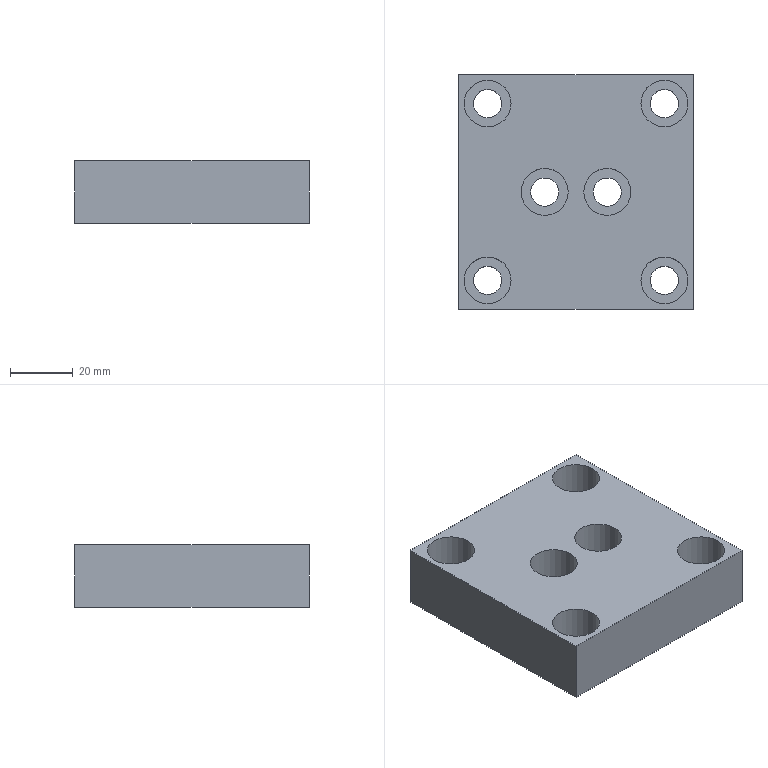Part | NX | features solid 2 | 1 solid | 24 faces | box 75 x 75 x 20 mm | volume 96271 mm3 | plane 12 | cylinder 12 | commonest cylinder face diameters 9 x6 15 x6
STEP:
#1=CARTESIAN_POINT('',(8.75,-278.25,320.));
#2=VERTEX_POINT('',#1);
#3=CARTESIAN_POINT('',(13.25,-278.25,320.));
#4=DIRECTION('',(0.,0.,-1.));
#5=DIRECTION('',(-1.,0.,0.));
#6=AXIS2_PLACEMENT_3D('',#3,#4,#5);
#7=CIRCLE('',#6,4.5);
#8=EDGE_CURVE('',#2,#2,#7,.F.);
#9=ORIENTED_EDGE('',*,*,#8,.T.);
#10=EDGE_LOOP('',(#9));
#11=FACE_BOUND('',#10,.T.);
#12=CARTESIAN_POINT('',(8.75,-221.75,320.));
#13=VERTEX_POINT('',#12);
#14=CARTESIAN_POINT('',(13.25,-221.75,320.));
#15=DIRECTION('',(0.,0.,-1.));
#16=DIRECTION('',(-1.,0.,0.));
#17=AXIS2_PLACEMENT_3D('',#14,#15,#16);
#18=CIRCLE('',#17,4.5);
#19=EDGE_CURVE('',#13,#13,#18,.F.);
#20=ORIENTED_EDGE('',*,*,#19,.T.);
#21=EDGE_LOOP('',(#20));
#22=FACE_BOUND('',#21,.T.);
#23=CARTESIAN_POINT('',(-47.75,-278.25,320.));
#24=VERTEX_POINT('',#23);
#25=CARTESIAN_POINT('',(-43.25,-278.25,320.));
#26=DIRECTION('',(0.,0.,-1.));
#27=DIRECTION('',(-1.,0.,0.));
#28=AXIS2_PLACEMENT_3D('',#25,#26,#27);
#29=CIRCLE('',#28,4.5);
#30=EDGE_CURVE('',#24,#24,#29,.F.);
#31=ORIENTED_EDGE('',*,*,#30,.T.);
#32=EDGE_LOOP('',(#31));
#33=FACE_BOUND('',#32,.T.);
#34=CARTESIAN_POINT('',(-47.75,-221.75,320.));
#35=VERTEX_POINT('',#34);
#36=CARTESIAN_POINT('',(-43.25,-221.75,320.));
#37=DIRECTION('',(0.,0.,-1.));
#38=DIRECTION('',(-1.,0.,0.));
#39=AXIS2_PLACEMENT_3D('',#36,#37,#38);
#40=CIRCLE('',#39,4.5);
#41=EDGE_CURVE('',#35,#35,#40,.F.);
#42=ORIENTED_EDGE('',*,*,#41,.T.);
#43=EDGE_LOOP('',(#42));
#44=FACE_BOUND('',#43,.T.);
#45=CARTESIAN_POINT('',(-9.5,-250.,320.));
#46=VERTEX_POINT('',#45);
#47=CARTESIAN_POINT('',(-5.,-250.,320.));
#48=DIRECTION('',(0.,0.,-1.));
#49=DIRECTION('',(-1.,0.,0.));
#50=AXIS2_PLACEMENT_3D('',#47,#48,#49);
#51=CIRCLE('',#50,4.5);
#52=EDGE_CURVE('',#46,#46,#51,.F.);
#53=ORIENTED_EDGE('',*,*,#52,.T.);
#54=EDGE_LOOP('',(#53));
#55=FACE_BOUND('',#54,.T.);
#56=CARTESIAN_POINT('',(-29.5,-250.,320.));
#57=VERTEX_POINT('',#56);
#58=CARTESIAN_POINT('',(-25.,-250.,320.));
#59=DIRECTION('',(0.,0.,-1.));
#60=DIRECTION('',(-1.,0.,0.));
#61=AXIS2_PLACEMENT_3D('',#58,#59,#60);
#62=CIRCLE('',#61,4.5);
#63=EDGE_CURVE('',#57,#57,#62,.F.);
#64=ORIENTED_EDGE('',*,*,#63,.T.);
#65=EDGE_LOOP('',(#64));
#66=FACE_BOUND('',#65,.T.);
#67=CARTESIAN_POINT('',(-52.5,-212.5,320.));
#68=VERTEX_POINT('',#67);
#69=CARTESIAN_POINT('',(22.5,-212.5,320.));
#70=VERTEX_POINT('',#69);
#71=CARTESIAN_POINT('',(-52.5,-212.5,320.));
#72=DIRECTION('',(-1.,0.,0.));
#73=VECTOR('',#72,1000.);
#74=LINE('',#71,#73);
#75=EDGE_CURVE('',#68,#70,#74,.F.);
#76=ORIENTED_EDGE('',*,*,#75,.T.);
#77=CARTESIAN_POINT('',(22.5,-287.5,320.));
#78=VERTEX_POINT('',#77);
#79=CARTESIAN_POINT('',(22.5,-212.5,320.));
#80=DIRECTION('',(0.,1.,0.));
#81=VECTOR('',#80,1000.);
#82=LINE('',#79,#81);
#83=EDGE_CURVE('',#70,#78,#82,.F.);
#84=ORIENTED_EDGE('',*,*,#83,.T.);
#85=CARTESIAN_POINT('',(-52.5,-287.5,320.));
#86=VERTEX_POINT('',#85);
#87=CARTESIAN_POINT('',(-52.5,-287.5,320.));
#88=DIRECTION('',(-1.,0.,0.));
#89=VECTOR('',#88,1000.);
#90=LINE('',#87,#89);
#91=EDGE_CURVE('',#86,#78,#90,.F.);
#92=ORIENTED_EDGE('',*,*,#91,.F.);
#93=CARTESIAN_POINT('',(-52.5,-212.5,320.));
#94=DIRECTION('',(0.,-1.,0.));
#95=VECTOR('',#94,1000.);
#96=LINE('',#93,#95);
#97=EDGE_CURVE('',#68,#86,#96,.T.);
#98=ORIENTED_EDGE('',*,*,#97,.F.);
#99=EDGE_LOOP('',(#76,#84,#92,#98));
#100=FACE_BOUND('',#99,.T.);
#101=CARTESIAN_POINT('',(-52.5,-212.5,320.));
#102=DIRECTION('',(0.,0.,-1.));
#103=DIRECTION('',(0.,-1.,0.));
#104=AXIS2_PLACEMENT_3D('',#101,#102,#103);
#105=PLANE('',#104);
#106=ADVANCED_FACE('',(#11,#22,#33,#44,#55,#66,#100),#105,.T.);
#107=ORIENTED_EDGE('',*,*,#91,.T.);
#108=CARTESIAN_POINT('',(22.5,-287.5,340.));
#109=VERTEX_POINT('',#108);
#110=CARTESIAN_POINT('',(22.5,-287.5,320.));
#111=DIRECTION('',(0.,0.,1.));
#112=VECTOR('',#111,1000.);
#113=LINE('',#110,#112);
#114=EDGE_CURVE('',#78,#109,#113,.T.);
#115=ORIENTED_EDGE('',*,*,#114,.T.);
#116=CARTESIAN_POINT('',(-52.5,-287.5,340.));
#117=VERTEX_POINT('',#116);
#118=CARTESIAN_POINT('',(-52.5,-287.5,340.));
#119=DIRECTION('',(-1.,0.,0.));
#120=VECTOR('',#119,1000.);
#121=LINE('',#118,#120);
#122=EDGE_CURVE('',#117,#109,#121,.F.);
#123=ORIENTED_EDGE('',*,*,#122,.F.);
#124=CARTESIAN_POINT('',(-52.5,-287.5,320.));
#125=DIRECTION('',(0.,0.,1.));
#126=VECTOR('',#125,1000.);
#127=LINE('',#124,#126);
#128=EDGE_CURVE('',#86,#117,#127,.T.);
#129=ORIENTED_EDGE('',*,*,#128,.F.);
#130=EDGE_LOOP('',(#107,#115,#123,#129));
#131=FACE_BOUND('',#130,.T.);
#132=CARTESIAN_POINT('',(-52.5,-287.5,320.));
#133=DIRECTION('',(0.,-1.,0.));
#134=DIRECTION('',(0.,0.,1.));
#135=AXIS2_PLACEMENT_3D('',#132,#133,#134);
#136=PLANE('',#135);
#137=ADVANCED_FACE('',(#131),#136,.T.);
#138=CARTESIAN_POINT('',(5.75,-278.25,340.));
#139=VERTEX_POINT('',#138);
#140=CARTESIAN_POINT('',(13.25,-278.25,340.));
#141=DIRECTION('',(0.,0.,-1.));
#142=DIRECTION('',(-1.,0.,0.));
#143=AXIS2_PLACEMENT_3D('',#140,#141,#142);
#144=CIRCLE('',#143,7.5);
#145=EDGE_CURVE('',#139,#139,#144,.T.);
#146=ORIENTED_EDGE('',*,*,#145,.T.);
#147=EDGE_LOOP('',(#146));
#148=FACE_BOUND('',#147,.T.);
#149=CARTESIAN_POINT('',(5.75,-221.75,340.));
#150=VERTEX_POINT('',#149);
#151=CARTESIAN_POINT('',(13.25,-221.75,340.));
#152=DIRECTION('',(0.,0.,-1.));
#153=DIRECTION('',(-1.,0.,0.));
#154=AXIS2_PLACEMENT_3D('',#151,#152,#153);
#155=CIRCLE('',#154,7.5);
#156=EDGE_CURVE('',#150,#150,#155,.T.);
#157=ORIENTED_EDGE('',*,*,#156,.T.);
#158=EDGE_LOOP('',(#157));
#159=FACE_BOUND('',#158,.T.);
#160=CARTESIAN_POINT('',(-50.75,-278.25,340.));
#161=VERTEX_POINT('',#160);
#162=CARTESIAN_POINT('',(-43.25,-278.25,340.));
#163=DIRECTION('',(0.,0.,-1.));
#164=DIRECTION('',(-1.,0.,0.));
#165=AXIS2_PLACEMENT_3D('',#162,#163,#164);
#166=CIRCLE('',#165,7.5);
#167=EDGE_CURVE('',#161,#161,#166,.T.);
#168=ORIENTED_EDGE('',*,*,#167,.T.);
#169=EDGE_LOOP('',(#168));
#170=FACE_BOUND('',#169,.T.);
#171=CARTESIAN_POINT('',(-50.75,-221.75,340.));
#172=VERTEX_POINT('',#171);
#173=CARTESIAN_POINT('',(-43.25,-221.75,340.));
#174=DIRECTION('',(0.,0.,-1.));
#175=DIRECTION('',(-1.,0.,0.));
#176=AXIS2_PLACEMENT_3D('',#173,#174,#175);
#177=CIRCLE('',#176,7.5);
#178=EDGE_CURVE('',#172,#172,#177,.T.);
#179=ORIENTED_EDGE('',*,*,#178,.T.);
#180=EDGE_LOOP('',(#179));
#181=FACE_BOUND('',#180,.T.);
#182=CARTESIAN_POINT('',(-12.5,-250.,340.));
#183=VERTEX_POINT('',#182);
#184=CARTESIAN_POINT('',(-5.,-250.,340.));
#185=DIRECTION('',(0.,0.,-1.));
#186=DIRECTION('',(-1.,0.,0.));
#187=AXIS2_PLACEMENT_3D('',#184,#185,#186);
#188=CIRCLE('',#187,7.5);
#189=EDGE_CURVE('',#183,#183,#188,.T.);
#190=ORIENTED_EDGE('',*,*,#189,.T.);
#191=EDGE_LOOP('',(#190));
#192=FACE_BOUND('',#191,.T.);
#193=CARTESIAN_POINT('',(-32.5,-250.,340.));
#194=VERTEX_POINT('',#193);
#195=CARTESIAN_POINT('',(-25.,-250.,340.));
#196=DIRECTION('',(0.,0.,-1.));
#197=DIRECTION('',(-1.,0.,0.));
#198=AXIS2_PLACEMENT_3D('',#195,#196,#197);
#199=CIRCLE('',#198,7.5);
#200=EDGE_CURVE('',#194,#194,#199,.T.);
#201=ORIENTED_EDGE('',*,*,#200,.T.);
#202=EDGE_LOOP('',(#201));
#203=FACE_BOUND('',#202,.T.);
#204=ORIENTED_EDGE('',*,*,#122,.T.);
#205=CARTESIAN_POINT('',(22.5,-212.5,340.));
#206=VERTEX_POINT('',#205);
#207=CARTESIAN_POINT('',(22.5,-212.5,340.));
#208=DIRECTION('',(0.,-1.,0.));
#209=VECTOR('',#208,1000.);
#210=LINE('',#207,#209);
#211=EDGE_CURVE('',#206,#109,#210,.T.);
#212=ORIENTED_EDGE('',*,*,#211,.F.);
#213=CARTESIAN_POINT('',(-52.5,-212.5,340.));
#214=VERTEX_POINT('',#213);
#215=CARTESIAN_POINT('',(-52.5,-212.5,340.));
#216=DIRECTION('',(1.,0.,0.));
#217=VECTOR('',#216,1000.);
#218=LINE('',#215,#217);
#219=EDGE_CURVE('',#214,#206,#218,.T.);
#220=ORIENTED_EDGE('',*,*,#219,.F.);
#221=CARTESIAN_POINT('',(-52.5,-212.5,340.));
#222=DIRECTION('',(0.,-1.,0.));
#223=VECTOR('',#222,1000.);
#224=LINE('',#221,#223);
#225=EDGE_CURVE('',#214,#117,#224,.T.);
#226=ORIENTED_EDGE('',*,*,#225,.T.);
#227=EDGE_LOOP('',(#204,#212,#220,#226));
#228=FACE_BOUND('',#227,.T.);
#229=CARTESIAN_POINT('',(-52.5,-212.5,340.));
#230=DIRECTION('',(0.,0.,-1.));
#231=DIRECTION('',(0.,-1.,0.));
#232=AXIS2_PLACEMENT_3D('',#229,#230,#231);
#233=PLANE('',#232);
#234=ADVANCED_FACE('',(#148,#159,#170,#181,#192,#203,#228),#233,.F.);
#235=CARTESIAN_POINT('',(-52.5,-212.5,320.));
#236=DIRECTION('',(0.,0.,1.));
#237=VECTOR('',#236,1000.);
#238=LINE('',#235,#237);
#239=EDGE_CURVE('',#68,#214,#238,.T.);
#240=ORIENTED_EDGE('',*,*,#239,.T.);
#241=ORIENTED_EDGE('',*,*,#219,.T.);
#242=CARTESIAN_POINT('',(22.5,-212.5,320.));
#243=DIRECTION('',(0.,0.,1.));
#244=VECTOR('',#243,1000.);
#245=LINE('',#242,#244);
#246=EDGE_CURVE('',#70,#206,#245,.T.);
#247=ORIENTED_EDGE('',*,*,#246,.F.);
#248=ORIENTED_EDGE('',*,*,#75,.F.);
#249=EDGE_LOOP('',(#240,#241,#247,#248));
#250=FACE_BOUND('',#249,.T.);
#251=CARTESIAN_POINT('',(-52.5,-212.5,320.));
#252=DIRECTION('',(0.,-1.,0.));
#253=DIRECTION('',(0.,0.,1.));
#254=AXIS2_PLACEMENT_3D('',#251,#252,#253);
#255=PLANE('',#254);
#256=ADVANCED_FACE('',(#250),#255,.F.);
#257=ORIENTED_EDGE('',*,*,#211,.T.);
#258=ORIENTED_EDGE('',*,*,#114,.F.);
#259=ORIENTED_EDGE('',*,*,#83,.F.);
#260=ORIENTED_EDGE('',*,*,#246,.T.);
#261=EDGE_LOOP('',(#257,#258,#259,#260));
#262=FACE_BOUND('',#261,.T.);
#263=CARTESIAN_POINT('',(22.5,-212.5,320.));
#264=DIRECTION('',(-1.,0.,0.));
#265=DIRECTION('',(0.,0.,1.));
#266=AXIS2_PLACEMENT_3D('',#263,#264,#265);
#267=PLANE('',#266);
#268=ADVANCED_FACE('',(#262),#267,.F.);
#269=ORIENTED_EDGE('',*,*,#225,.F.);
#270=ORIENTED_EDGE('',*,*,#239,.F.);
#271=ORIENTED_EDGE('',*,*,#97,.T.);
#272=ORIENTED_EDGE('',*,*,#128,.T.);
#273=EDGE_LOOP('',(#269,#270,#271,#272));
#274=FACE_BOUND('',#273,.T.);
#275=CARTESIAN_POINT('',(-52.5,-212.5,320.));
#276=DIRECTION('',(-1.,0.,0.));
#277=DIRECTION('',(0.,0.,1.));
#278=AXIS2_PLACEMENT_3D('',#275,#276,#277);
#279=PLANE('',#278);
#280=ADVANCED_FACE('',(#274),#279,.T.);
#281=CARTESIAN_POINT('',(-29.5,-250.,326.));
#282=VERTEX_POINT('',#281);
#283=CARTESIAN_POINT('',(-25.,-250.,326.));
#284=DIRECTION('',(0.,0.,-1.));
#285=DIRECTION('',(-1.,0.,0.));
#286=AXIS2_PLACEMENT_3D('',#283,#284,#285);
#287=CIRCLE('',#286,4.5);
#288=EDGE_CURVE('',#282,#282,#287,.T.);
#289=ORIENTED_EDGE('',*,*,#288,.F.);
#290=EDGE_LOOP('',(#289));
#291=FACE_BOUND('',#290,.T.);
#292=ORIENTED_EDGE('',*,*,#63,.F.);
#293=EDGE_LOOP('',(#292));
#294=FACE_BOUND('',#293,.T.);
#295=CARTESIAN_POINT('',(-25.,-250.,290.));
#296=DIRECTION('',(0.,0.,-1.));
#297=DIRECTION('',(-1.,0.,0.));
#298=AXIS2_PLACEMENT_3D('',#295,#296,#297);
#299=CYLINDRICAL_SURFACE('',#298,4.5);
#300=ADVANCED_FACE('',(#291,#294),#299,.F.);
#301=ORIENTED_EDGE('',*,*,#288,.T.);
#302=EDGE_LOOP('',(#301));
#303=FACE_BOUND('',#302,.T.);
#304=CARTESIAN_POINT('',(-32.5,-250.,326.));
#305=VERTEX_POINT('',#304);
#306=CARTESIAN_POINT('',(-25.,-250.,326.));
#307=DIRECTION('',(0.,0.,-1.));
#308=DIRECTION('',(-1.,0.,0.));
#309=AXIS2_PLACEMENT_3D('',#306,#307,#308);
#310=CIRCLE('',#309,7.5);
#311=EDGE_CURVE('',#305,#305,#310,.T.);
#312=ORIENTED_EDGE('',*,*,#311,.F.);
#313=EDGE_LOOP('',(#312));
#314=FACE_BOUND('',#313,.T.);
#315=CARTESIAN_POINT('',(-25.,-250.,326.));
#316=DIRECTION('',(0.,0.,-1.));
#317=DIRECTION('',(-1.,0.,0.));
#318=AXIS2_PLACEMENT_3D('',#315,#316,#317);
#319=PLANE('',#318);
#320=ADVANCED_FACE('',(#303,#314),#319,.F.);
#321=ORIENTED_EDGE('',*,*,#311,.T.);
#322=EDGE_LOOP('',(#321));
#323=FACE_BOUND('',#322,.T.);
#324=ORIENTED_EDGE('',*,*,#200,.F.);
#325=EDGE_LOOP('',(#324));
#326=FACE_BOUND('',#325,.T.);
#327=CARTESIAN_POINT('',(-25.,-250.,340.));
#328=DIRECTION('',(0.,0.,-1.));
#329=DIRECTION('',(-1.,0.,0.));
#330=AXIS2_PLACEMENT_3D('',#327,#328,#329);
#331=CYLINDRICAL_SURFACE('',#330,7.5);
#332=ADVANCED_FACE('',(#323,#326),#331,.F.);
#333=CARTESIAN_POINT('',(-9.5,-250.,326.));
#334=VERTEX_POINT('',#333);
#335=CARTESIAN_POINT('',(-5.,-250.,326.));
#336=DIRECTION('',(0.,0.,-1.));
#337=DIRECTION('',(-1.,0.,0.));
#338=AXIS2_PLACEMENT_3D('',#335,#336,#337);
#339=CIRCLE('',#338,4.5);
#340=EDGE_CURVE('',#334,#334,#339,.T.);
#341=ORIENTED_EDGE('',*,*,#340,.F.);
#342=EDGE_LOOP('',(#341));
#343=FACE_BOUND('',#342,.T.);
#344=ORIENTED_EDGE('',*,*,#52,.F.);
#345=EDGE_LOOP('',(#344));
#346=FACE_BOUND('',#345,.T.);
#347=CARTESIAN_POINT('',(-5.,-250.,290.));
#348=DIRECTION('',(0.,0.,-1.));
#349=DIRECTION('',(-1.,0.,0.));
#350=AXIS2_PLACEMENT_3D('',#347,#348,#349);
#351=CYLINDRICAL_SURFACE('',#350,4.5);
#352=ADVANCED_FACE('',(#343,#346),#351,.F.);
#353=ORIENTED_EDGE('',*,*,#340,.T.);
#354=EDGE_LOOP('',(#353));
#355=FACE_BOUND('',#354,.T.);
#356=CARTESIAN_POINT('',(-12.5,-250.,326.));
#357=VERTEX_POINT('',#356);
#358=CARTESIAN_POINT('',(-5.,-250.,326.));
#359=DIRECTION('',(0.,0.,-1.));
#360=DIRECTION('',(-1.,0.,0.));
#361=AXIS2_PLACEMENT_3D('',#358,#359,#360);
#362=CIRCLE('',#361,7.5);
#363=EDGE_CURVE('',#357,#357,#362,.T.);
#364=ORIENTED_EDGE('',*,*,#363,.F.);
#365=EDGE_LOOP('',(#364));
#366=FACE_BOUND('',#365,.T.);
#367=CARTESIAN_POINT('',(-5.,-250.,326.));
#368=DIRECTION('',(0.,0.,-1.));
#369=DIRECTION('',(-1.,0.,0.));
#370=AXIS2_PLACEMENT_3D('',#367,#368,#369);
#371=PLANE('',#370);
#372=ADVANCED_FACE('',(#355,#366),#371,.F.);
#373=ORIENTED_EDGE('',*,*,#363,.T.);
#374=EDGE_LOOP('',(#373));
#375=FACE_BOUND('',#374,.T.);
#376=ORIENTED_EDGE('',*,*,#189,.F.);
#377=EDGE_LOOP('',(#376));
#378=FACE_BOUND('',#377,.T.);
#379=CARTESIAN_POINT('',(-5.,-250.,340.));
#380=DIRECTION('',(0.,0.,-1.));
#381=DIRECTION('',(-1.,0.,0.));
#382=AXIS2_PLACEMENT_3D('',#379,#380,#381);
#383=CYLINDRICAL_SURFACE('',#382,7.5);
#384=ADVANCED_FACE('',(#375,#378),#383,.F.);
#385=CARTESIAN_POINT('',(-47.75,-221.75,328.));
#386=VERTEX_POINT('',#385);
#387=CARTESIAN_POINT('',(-43.25,-221.75,328.));
#388=DIRECTION('',(0.,0.,-1.));
#389=DIRECTION('',(-1.,0.,0.));
#390=AXIS2_PLACEMENT_3D('',#387,#388,#389);
#391=CIRCLE('',#390,4.5);
#392=EDGE_CURVE('',#386,#386,#391,.T.);
#393=ORIENTED_EDGE('',*,*,#392,.F.);
#394=EDGE_LOOP('',(#393));
#395=FACE_BOUND('',#394,.T.);
#396=ORIENTED_EDGE('',*,*,#41,.F.);
#397=EDGE_LOOP('',(#396));
#398=FACE_BOUND('',#397,.T.);
#399=CARTESIAN_POINT('',(-43.25,-221.75,290.));
#400=DIRECTION('',(0.,0.,-1.));
#401=DIRECTION('',(-1.,0.,0.));
#402=AXIS2_PLACEMENT_3D('',#399,#400,#401);
#403=CYLINDRICAL_SURFACE('',#402,4.5);
#404=ADVANCED_FACE('',(#395,#398),#403,.F.);
#405=ORIENTED_EDGE('',*,*,#392,.T.);
#406=EDGE_LOOP('',(#405));
#407=FACE_BOUND('',#406,.T.);
#408=CARTESIAN_POINT('',(-50.75,-221.75,328.));
#409=VERTEX_POINT('',#408);
#410=CARTESIAN_POINT('',(-43.25,-221.75,328.));
#411=DIRECTION('',(0.,0.,-1.));
#412=DIRECTION('',(-1.,0.,0.));
#413=AXIS2_PLACEMENT_3D('',#410,#411,#412);
#414=CIRCLE('',#413,7.5);
#415=EDGE_CURVE('',#409,#409,#414,.T.);
#416=ORIENTED_EDGE('',*,*,#415,.F.);
#417=EDGE_LOOP('',(#416));
#418=FACE_BOUND('',#417,.T.);
#419=CARTESIAN_POINT('',(-43.25,-221.75,328.));
#420=DIRECTION('',(0.,0.,-1.));
#421=DIRECTION('',(-1.,0.,0.));
#422=AXIS2_PLACEMENT_3D('',#419,#420,#421);
#423=PLANE('',#422);
#424=ADVANCED_FACE('',(#407,#418),#423,.F.);
#425=ORIENTED_EDGE('',*,*,#415,.T.);
#426=EDGE_LOOP('',(#425));
#427=FACE_BOUND('',#426,.T.);
#428=ORIENTED_EDGE('',*,*,#178,.F.);
#429=EDGE_LOOP('',(#428));
#430=FACE_BOUND('',#429,.T.);
#431=CARTESIAN_POINT('',(-43.25,-221.75,340.));
#432=DIRECTION('',(0.,0.,-1.));
#433=DIRECTION('',(-1.,0.,0.));
#434=AXIS2_PLACEMENT_3D('',#431,#432,#433);
#435=CYLINDRICAL_SURFACE('',#434,7.5);
#436=ADVANCED_FACE('',(#427,#430),#435,.F.);
#437=CARTESIAN_POINT('',(-47.75,-278.25,328.));
#438=VERTEX_POINT('',#437);
#439=CARTESIAN_POINT('',(-43.25,-278.25,328.));
#440=DIRECTION('',(0.,0.,-1.));
#441=DIRECTION('',(-1.,0.,0.));
#442=AXIS2_PLACEMENT_3D('',#439,#440,#441);
#443=CIRCLE('',#442,4.5);
#444=EDGE_CURVE('',#438,#438,#443,.T.);
#445=ORIENTED_EDGE('',*,*,#444,.F.);
#446=EDGE_LOOP('',(#445));
#447=FACE_BOUND('',#446,.T.);
#448=ORIENTED_EDGE('',*,*,#30,.F.);
#449=EDGE_LOOP('',(#448));
#450=FACE_BOUND('',#449,.T.);
#451=CARTESIAN_POINT('',(-43.25,-278.25,290.));
#452=DIRECTION('',(0.,0.,-1.));
#453=DIRECTION('',(-1.,0.,0.));
#454=AXIS2_PLACEMENT_3D('',#451,#452,#453);
#455=CYLINDRICAL_SURFACE('',#454,4.5);
#456=ADVANCED_FACE('',(#447,#450),#455,.F.);
#457=ORIENTED_EDGE('',*,*,#444,.T.);
#458=EDGE_LOOP('',(#457));
#459=FACE_BOUND('',#458,.T.);
#460=CARTESIAN_POINT('',(-50.75,-278.25,328.));
#461=VERTEX_POINT('',#460);
#462=CARTESIAN_POINT('',(-43.25,-278.25,328.));
#463=DIRECTION('',(0.,0.,-1.));
#464=DIRECTION('',(-1.,0.,0.));
#465=AXIS2_PLACEMENT_3D('',#462,#463,#464);
#466=CIRCLE('',#465,7.5);
#467=EDGE_CURVE('',#461,#461,#466,.T.);
#468=ORIENTED_EDGE('',*,*,#467,.F.);
#469=EDGE_LOOP('',(#468));
#470=FACE_BOUND('',#469,.T.);
#471=CARTESIAN_POINT('',(-43.25,-278.25,328.));
#472=DIRECTION('',(0.,0.,-1.));
#473=DIRECTION('',(-1.,0.,0.));
#474=AXIS2_PLACEMENT_3D('',#471,#472,#473);
#475=PLANE('',#474);
#476=ADVANCED_FACE('',(#459,#470),#475,.F.);
#477=ORIENTED_EDGE('',*,*,#467,.T.);
#478=EDGE_LOOP('',(#477));
#479=FACE_BOUND('',#478,.T.);
#480=ORIENTED_EDGE('',*,*,#167,.F.);
#481=EDGE_LOOP('',(#480));
#482=FACE_BOUND('',#481,.T.);
#483=CARTESIAN_POINT('',(-43.25,-278.25,340.));
#484=DIRECTION('',(0.,0.,-1.));
#485=DIRECTION('',(-1.,0.,0.));
#486=AXIS2_PLACEMENT_3D('',#483,#484,#485);
#487=CYLINDRICAL_SURFACE('',#486,7.5);
#488=ADVANCED_FACE('',(#479,#482),#487,.F.);
#489=CARTESIAN_POINT('',(8.75,-221.75,328.));
#490=VERTEX_POINT('',#489);
#491=CARTESIAN_POINT('',(13.25,-221.75,328.));
#492=DIRECTION('',(0.,0.,-1.));
#493=DIRECTION('',(-1.,0.,0.));
#494=AXIS2_PLACEMENT_3D('',#491,#492,#493);
#495=CIRCLE('',#494,4.5);
#496=EDGE_CURVE('',#490,#490,#495,.T.);
#497=ORIENTED_EDGE('',*,*,#496,.F.);
#498=EDGE_LOOP('',(#497));
#499=FACE_BOUND('',#498,.T.);
#500=ORIENTED_EDGE('',*,*,#19,.F.);
#501=EDGE_LOOP('',(#500));
#502=FACE_BOUND('',#501,.T.);
#503=CARTESIAN_POINT('',(13.25,-221.75,290.));
#504=DIRECTION('',(0.,0.,-1.));
#505=DIRECTION('',(-1.,0.,0.));
#506=AXIS2_PLACEMENT_3D('',#503,#504,#505);
#507=CYLINDRICAL_SURFACE('',#506,4.5);
#508=ADVANCED_FACE('',(#499,#502),#507,.F.);
#509=ORIENTED_EDGE('',*,*,#496,.T.);
#510=EDGE_LOOP('',(#509));
#511=FACE_BOUND('',#510,.T.);
#512=CARTESIAN_POINT('',(5.75,-221.75,328.));
#513=VERTEX_POINT('',#512);
#514=CARTESIAN_POINT('',(13.25,-221.75,328.));
#515=DIRECTION('',(0.,0.,-1.));
#516=DIRECTION('',(-1.,0.,0.));
#517=AXIS2_PLACEMENT_3D('',#514,#515,#516);
#518=CIRCLE('',#517,7.5);
#519=EDGE_CURVE('',#513,#513,#518,.T.);
#520=ORIENTED_EDGE('',*,*,#519,.F.);
#521=EDGE_LOOP('',(#520));
#522=FACE_BOUND('',#521,.T.);
#523=CARTESIAN_POINT('',(13.25,-221.75,328.));
#524=DIRECTION('',(0.,0.,-1.));
#525=DIRECTION('',(-1.,0.,0.));
#526=AXIS2_PLACEMENT_3D('',#523,#524,#525);
#527=PLANE('',#526);
#528=ADVANCED_FACE('',(#511,#522),#527,.F.);
#529=ORIENTED_EDGE('',*,*,#519,.T.);
#530=EDGE_LOOP('',(#529));
#531=FACE_BOUND('',#530,.T.);
#532=ORIENTED_EDGE('',*,*,#156,.F.);
#533=EDGE_LOOP('',(#532));
#534=FACE_BOUND('',#533,.T.);
#535=CARTESIAN_POINT('',(13.25,-221.75,340.));
#536=DIRECTION('',(0.,0.,-1.));
#537=DIRECTION('',(-1.,0.,0.));
#538=AXIS2_PLACEMENT_3D('',#535,#536,#537);
#539=CYLINDRICAL_SURFACE('',#538,7.5);
#540=ADVANCED_FACE('',(#531,#534),#539,.F.);
#541=CARTESIAN_POINT('',(8.75,-278.25,328.));
#542=VERTEX_POINT('',#541);
#543=CARTESIAN_POINT('',(13.25,-278.25,328.));
#544=DIRECTION('',(0.,0.,-1.));
#545=DIRECTION('',(-1.,0.,0.));
#546=AXIS2_PLACEMENT_3D('',#543,#544,#545);
#547=CIRCLE('',#546,4.5);
#548=EDGE_CURVE('',#542,#542,#547,.T.);
#549=ORIENTED_EDGE('',*,*,#548,.F.);
#550=EDGE_LOOP('',(#549));
#551=FACE_BOUND('',#550,.T.);
#552=ORIENTED_EDGE('',*,*,#8,.F.);
#553=EDGE_LOOP('',(#552));
#554=FACE_BOUND('',#553,.T.);
#555=CARTESIAN_POINT('',(13.25,-278.25,290.));
#556=DIRECTION('',(0.,0.,-1.));
#557=DIRECTION('',(-1.,0.,0.));
#558=AXIS2_PLACEMENT_3D('',#555,#556,#557);
#559=CYLINDRICAL_SURFACE('',#558,4.5);
#560=ADVANCED_FACE('',(#551,#554),#559,.F.);
#561=ORIENTED_EDGE('',*,*,#548,.T.);
#562=EDGE_LOOP('',(#561));
#563=FACE_BOUND('',#562,.T.);
#564=CARTESIAN_POINT('',(5.75,-278.25,328.));
#565=VERTEX_POINT('',#564);
#566=CARTESIAN_POINT('',(13.25,-278.25,328.));
#567=DIRECTION('',(0.,0.,-1.));
#568=DIRECTION('',(-1.,0.,0.));
#569=AXIS2_PLACEMENT_3D('',#566,#567,#568);
#570=CIRCLE('',#569,7.5);
#571=EDGE_CURVE('',#565,#565,#570,.T.);
#572=ORIENTED_EDGE('',*,*,#571,.F.);
#573=EDGE_LOOP('',(#572));
#574=FACE_BOUND('',#573,.T.);
#575=CARTESIAN_POINT('',(13.25,-278.25,328.));
#576=DIRECTION('',(0.,0.,-1.));
#577=DIRECTION('',(-1.,0.,0.));
#578=AXIS2_PLACEMENT_3D('',#575,#576,#577);
#579=PLANE('',#578);
#580=ADVANCED_FACE('',(#563,#574),#579,.F.);
#581=ORIENTED_EDGE('',*,*,#571,.T.);
#582=EDGE_LOOP('',(#581));
#583=FACE_BOUND('',#582,.T.);
#584=ORIENTED_EDGE('',*,*,#145,.F.);
#585=EDGE_LOOP('',(#584));
#586=FACE_BOUND('',#585,.T.);
#587=CARTESIAN_POINT('',(13.25,-278.25,340.));
#588=DIRECTION('',(0.,0.,-1.));
#589=DIRECTION('',(-1.,0.,0.));
#590=AXIS2_PLACEMENT_3D('',#587,#588,#589);
#591=CYLINDRICAL_SURFACE('',#590,7.5);
#592=ADVANCED_FACE('',(#583,#586),#591,.F.);
#593=CLOSED_SHELL('',(#106,#137,#234,#256,#268,#280,#300,#320,#332,#352,#372,#384,#404,#424,#436,#456,#476,#488,#508,#528,#540,#560,#580,#592));
#594=MANIFOLD_SOLID_BREP('',#593);
#595=(LENGTH_UNIT()NAMED_UNIT(*)SI_UNIT(.MILLI.,.METRE.));
#596=UNCERTAINTY_MEASURE_WITH_UNIT(LENGTH_MEASURE(0.00001),#595,'','');
#597=(NAMED_UNIT(*)PLANE_ANGLE_UNIT()SI_UNIT($,.RADIAN.));
#598=(NAMED_UNIT(*)SI_UNIT($,.STERADIAN.)SOLID_ANGLE_UNIT());
#599=(GEOMETRIC_REPRESENTATION_CONTEXT(3)GLOBAL_UNCERTAINTY_ASSIGNED_CONTEXT((#596))GLOBAL_UNIT_ASSIGNED_CONTEXT((#595,#597,#598))REPRESENTATION_CONTEXT('',''));
#600=ADVANCED_BREP_SHAPE_REPRESENTATION('',(#594),#599);